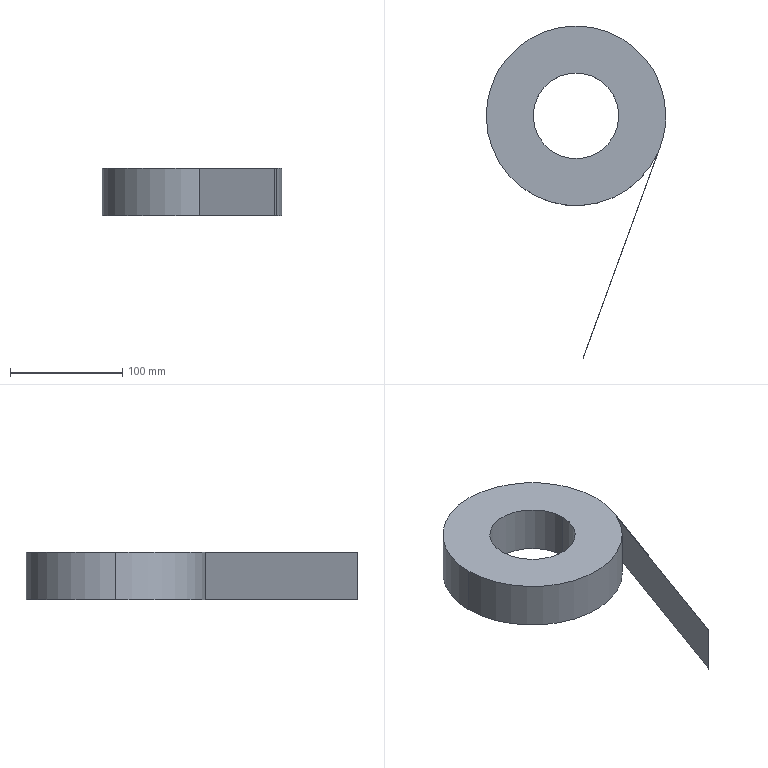Part | STEP file | 10000020479swp000-1 | 1 solid | 10 faces | box 160 x 295.688 x 42 mm | volume 654576 mm3 | cylinder 5 | plane 5 | commonest cylinder face diameters 160 x3 76.2 x2
STEP:
#1=CARTESIAN_POINT('',(-38.1,0.,30.));
#2=VERTEX_POINT('',#1);
#3=CARTESIAN_POINT('',(38.1,0.,30.));
#4=VERTEX_POINT('',#3);
#5=CARTESIAN_POINT('',(0.,0.,30.));
#6=DIRECTION('',(0.,0.,1.));
#7=DIRECTION('',(1.,0.,0.));
#8=AXIS2_PLACEMENT_3D('',#5,#6,#7);
#9=CIRCLE('',#8,38.1);
#10=EDGE_CURVE('',#2,#4,#9,.T.);
#11=ORIENTED_EDGE('',*,*,#10,.T.);
#12=CARTESIAN_POINT('',(38.1,0.,-12.));
#13=VERTEX_POINT('',#12);
#14=CARTESIAN_POINT('',(38.1,0.,30.));
#15=DIRECTION('',(0.,0.,-1.));
#16=VECTOR('',#15,1000.);
#17=LINE('',#14,#16);
#18=EDGE_CURVE('',#4,#13,#17,.T.);
#19=ORIENTED_EDGE('',*,*,#18,.T.);
#20=CARTESIAN_POINT('',(-38.1,0.,-12.));
#21=VERTEX_POINT('',#20);
#22=CARTESIAN_POINT('',(0.,0.,-12.));
#23=DIRECTION('',(0.,0.,1.));
#24=DIRECTION('',(1.,0.,0.));
#25=AXIS2_PLACEMENT_3D('',#22,#23,#24);
#26=CIRCLE('',#25,38.1);
#27=EDGE_CURVE('',#21,#13,#26,.T.);
#28=ORIENTED_EDGE('',*,*,#27,.F.);
#29=CARTESIAN_POINT('',(-38.1,0.,30.));
#30=DIRECTION('',(0.,0.,-1.));
#31=VECTOR('',#30,1000.);
#32=LINE('',#29,#31);
#33=EDGE_CURVE('',#2,#21,#32,.T.);
#34=ORIENTED_EDGE('',*,*,#33,.F.);
#35=EDGE_LOOP('',(#11,#19,#28,#34));
#36=FACE_OUTER_BOUND('',#35,.T.);
#37=CARTESIAN_POINT('',(0.,0.,30.));
#38=DIRECTION('',(0.,0.,-1.));
#39=DIRECTION('',(-1.,0.,0.));
#40=AXIS2_PLACEMENT_3D('',#37,#38,#39);
#41=CYLINDRICAL_SURFACE('',#40,38.1);
#42=ADVANCED_FACE('',(#36),#41,.F.);
#43=CARTESIAN_POINT('',(80.,0.,30.));
#44=VERTEX_POINT('',#43);
#45=CARTESIAN_POINT('',(-80.,0.,30.));
#46=VERTEX_POINT('',#45);
#47=CARTESIAN_POINT('',(0.,0.,30.));
#48=DIRECTION('',(0.,0.,1.));
#49=DIRECTION('',(1.,0.,0.));
#50=AXIS2_PLACEMENT_3D('',#47,#48,#49);
#51=CIRCLE('',#50,80.);
#52=EDGE_CURVE('',#44,#46,#51,.T.);
#53=ORIENTED_EDGE('',*,*,#52,.F.);
#54=CARTESIAN_POINT('',(80.,0.,-12.));
#55=VERTEX_POINT('',#54);
#56=CARTESIAN_POINT('',(80.,0.,30.));
#57=DIRECTION('',(0.,0.,-1.));
#58=VECTOR('',#57,1000.);
#59=LINE('',#56,#58);
#60=EDGE_CURVE('',#44,#55,#59,.T.);
#61=ORIENTED_EDGE('',*,*,#60,.T.);
#62=CARTESIAN_POINT('',(-80.,0.,-12.));
#63=VERTEX_POINT('',#62);
#64=CARTESIAN_POINT('',(0.,0.,-12.));
#65=DIRECTION('',(0.,0.,1.));
#66=DIRECTION('',(1.,0.,0.));
#67=AXIS2_PLACEMENT_3D('',#64,#65,#66);
#68=CIRCLE('',#67,80.);
#69=EDGE_CURVE('',#55,#63,#68,.T.);
#70=ORIENTED_EDGE('',*,*,#69,.T.);
#71=CARTESIAN_POINT('',(-80.,0.,30.));
#72=DIRECTION('',(0.,0.,-1.));
#73=VECTOR('',#72,1000.);
#74=LINE('',#71,#73);
#75=EDGE_CURVE('',#46,#63,#74,.T.);
#76=ORIENTED_EDGE('',*,*,#75,.F.);
#77=EDGE_LOOP('',(#53,#61,#70,#76));
#78=FACE_OUTER_BOUND('',#77,.T.);
#79=CARTESIAN_POINT('',(0.,0.,30.));
#80=DIRECTION('',(0.,0.,-1.));
#81=DIRECTION('',(-1.,0.,0.));
#82=AXIS2_PLACEMENT_3D('',#79,#80,#81);
#83=CYLINDRICAL_SURFACE('',#82,80.);
#84=ADVANCED_FACE('',(#78),#83,.T.);
#85=CARTESIAN_POINT('',(73.054,-32.606,30.));
#86=VERTEX_POINT('',#85);
#87=CARTESIAN_POINT('',(0.,0.,30.));
#88=DIRECTION('',(0.,0.,1.));
#89=DIRECTION('',(1.,0.,0.));
#90=AXIS2_PLACEMENT_3D('',#87,#88,#89);
#91=CIRCLE('',#90,80.);
#92=EDGE_CURVE('',#46,#86,#91,.T.);
#93=ORIENTED_EDGE('',*,*,#92,.F.);
#94=ORIENTED_EDGE('',*,*,#75,.T.);
#95=CARTESIAN_POINT('',(73.054,-32.606,-12.));
#96=VERTEX_POINT('',#95);
#97=CARTESIAN_POINT('',(0.,0.,-12.));
#98=DIRECTION('',(0.,0.,1.));
#99=DIRECTION('',(1.,0.,0.));
#100=AXIS2_PLACEMENT_3D('',#97,#98,#99);
#101=CIRCLE('',#100,80.);
#102=EDGE_CURVE('',#63,#96,#101,.T.);
#103=ORIENTED_EDGE('',*,*,#102,.T.);
#104=CARTESIAN_POINT('',(73.054,-32.606,30.));
#105=DIRECTION('',(0.,0.,1.));
#106=VECTOR('',#105,1000.);
#107=LINE('',#104,#106);
#108=EDGE_CURVE('',#96,#86,#107,.T.);
#109=ORIENTED_EDGE('',*,*,#108,.T.);
#110=EDGE_LOOP('',(#93,#94,#103,#109));
#111=FACE_OUTER_BOUND('',#110,.T.);
#112=CARTESIAN_POINT('',(0.,0.,30.));
#113=DIRECTION('',(0.,0.,-1.));
#114=DIRECTION('',(-1.,0.,0.));
#115=AXIS2_PLACEMENT_3D('',#112,#113,#114);
#116=CYLINDRICAL_SURFACE('',#115,80.);
#117=ADVANCED_FACE('',(#111),#116,.T.);
#118=ORIENTED_EDGE('',*,*,#60,.F.);
#119=CARTESIAN_POINT('',(75.175,-27.362,30.));
#120=VERTEX_POINT('',#119);
#121=CARTESIAN_POINT('',(0.,0.,30.));
#122=DIRECTION('',(0.,0.,1.));
#123=DIRECTION('',(1.,0.,0.));
#124=AXIS2_PLACEMENT_3D('',#121,#122,#123);
#125=CIRCLE('',#124,80.);
#126=EDGE_CURVE('',#120,#44,#125,.T.);
#127=ORIENTED_EDGE('',*,*,#126,.F.);
#128=CARTESIAN_POINT('',(75.175,-27.362,-12.));
#129=VERTEX_POINT('',#128);
#130=CARTESIAN_POINT('',(75.175,-27.362,-200.541));
#131=DIRECTION('',(0.,0.,1.));
#132=VECTOR('',#131,1000.);
#133=LINE('',#130,#132);
#134=EDGE_CURVE('',#129,#120,#133,.T.);
#135=ORIENTED_EDGE('',*,*,#134,.F.);
#136=CARTESIAN_POINT('',(0.,0.,-12.));
#137=DIRECTION('',(0.,0.,1.));
#138=DIRECTION('',(1.,0.,0.));
#139=AXIS2_PLACEMENT_3D('',#136,#137,#138);
#140=CIRCLE('',#139,80.);
#141=EDGE_CURVE('',#129,#55,#140,.T.);
#142=ORIENTED_EDGE('',*,*,#141,.T.);
#143=EDGE_LOOP('',(#118,#127,#135,#142));
#144=FACE_OUTER_BOUND('',#143,.T.);
#145=CARTESIAN_POINT('',(0.,0.,30.));
#146=DIRECTION('',(0.,0.,-1.));
#147=DIRECTION('',(-1.,0.,0.));
#148=AXIS2_PLACEMENT_3D('',#145,#146,#147);
#149=CYLINDRICAL_SURFACE('',#148,80.);
#150=ADVANCED_FACE('',(#144),#149,.T.);
#151=CARTESIAN_POINT('',(6.63,-215.688,30.));
#152=VERTEX_POINT('',#151);
#153=CARTESIAN_POINT('',(75.175,-27.362,30.));
#154=DIRECTION('',(-0.342,-0.9397,0.));
#155=VECTOR('',#154,1000.);
#156=LINE('',#153,#155);
#157=EDGE_CURVE('',#120,#152,#156,.T.);
#158=ORIENTED_EDGE('',*,*,#157,.F.);
#159=ORIENTED_EDGE('',*,*,#126,.T.);
#160=ORIENTED_EDGE('',*,*,#52,.T.);
#161=ORIENTED_EDGE('',*,*,#92,.T.);
#162=CARTESIAN_POINT('',(6.442,-215.619,30.));
#163=VERTEX_POINT('',#162);
#164=CARTESIAN_POINT('',(74.987,-27.293,30.));
#165=DIRECTION('',(-0.342,-0.9397,0.));
#166=VECTOR('',#165,1000.);
#167=LINE('',#164,#166);
#168=EDGE_CURVE('',#86,#163,#167,.T.);
#169=ORIENTED_EDGE('',*,*,#168,.T.);
#170=CARTESIAN_POINT('',(6.63,-215.688,30.));
#171=DIRECTION('',(-0.9397,0.342,0.));
#172=VECTOR('',#171,1000.);
#173=LINE('',#170,#172);
#174=EDGE_CURVE('',#152,#163,#173,.T.);
#175=ORIENTED_EDGE('',*,*,#174,.F.);
#176=EDGE_LOOP('',(#158,#159,#160,#161,#169,#175));
#177=FACE_OUTER_BOUND('',#176,.T.);
#178=ORIENTED_EDGE('',*,*,#10,.F.);
#179=CARTESIAN_POINT('',(0.,0.,30.));
#180=DIRECTION('',(0.,0.,1.));
#181=DIRECTION('',(1.,0.,0.));
#182=AXIS2_PLACEMENT_3D('',#179,#180,#181);
#183=CIRCLE('',#182,38.1);
#184=EDGE_CURVE('',#4,#2,#183,.T.);
#185=ORIENTED_EDGE('',*,*,#184,.F.);
#186=EDGE_LOOP('',(#178,#185));
#187=FACE_BOUND('',#186,.T.);
#188=CARTESIAN_POINT('',(0.,0.,30.));
#189=DIRECTION('',(0.,0.,1.));
#190=DIRECTION('',(1.,0.,0.));
#191=AXIS2_PLACEMENT_3D('',#188,#189,#190);
#192=PLANE('',#191);
#193=ADVANCED_FACE('',(#177,#187),#192,.T.);
#194=ORIENTED_EDGE('',*,*,#141,.F.);
#195=CARTESIAN_POINT('',(6.63,-215.688,-12.));
#196=VERTEX_POINT('',#195);
#197=CARTESIAN_POINT('',(75.175,-27.362,-12.));
#198=DIRECTION('',(0.342,0.9397,0.));
#199=VECTOR('',#198,1000.);
#200=LINE('',#197,#199);
#201=EDGE_CURVE('',#196,#129,#200,.T.);
#202=ORIENTED_EDGE('',*,*,#201,.F.);
#203=CARTESIAN_POINT('',(6.442,-215.619,-12.));
#204=VERTEX_POINT('',#203);
#205=CARTESIAN_POINT('',(6.63,-215.688,-12.));
#206=DIRECTION('',(0.9397,-0.342,0.));
#207=VECTOR('',#206,1000.);
#208=LINE('',#205,#207);
#209=EDGE_CURVE('',#204,#196,#208,.T.);
#210=ORIENTED_EDGE('',*,*,#209,.F.);
#211=CARTESIAN_POINT('',(74.987,-27.293,-12.));
#212=DIRECTION('',(0.342,0.9397,0.));
#213=VECTOR('',#212,1000.);
#214=LINE('',#211,#213);
#215=EDGE_CURVE('',#204,#96,#214,.T.);
#216=ORIENTED_EDGE('',*,*,#215,.T.);
#217=ORIENTED_EDGE('',*,*,#102,.F.);
#218=ORIENTED_EDGE('',*,*,#69,.F.);
#219=EDGE_LOOP('',(#194,#202,#210,#216,#217,#218));
#220=FACE_OUTER_BOUND('',#219,.T.);
#221=ORIENTED_EDGE('',*,*,#27,.T.);
#222=CARTESIAN_POINT('',(0.,0.,-12.));
#223=DIRECTION('',(0.,0.,1.));
#224=DIRECTION('',(1.,0.,0.));
#225=AXIS2_PLACEMENT_3D('',#222,#223,#224);
#226=CIRCLE('',#225,38.1);
#227=EDGE_CURVE('',#13,#21,#226,.T.);
#228=ORIENTED_EDGE('',*,*,#227,.T.);
#229=EDGE_LOOP('',(#221,#228));
#230=FACE_BOUND('',#229,.T.);
#231=CARTESIAN_POINT('',(0.,0.,-12.));
#232=DIRECTION('',(0.,0.,1.));
#233=DIRECTION('',(1.,0.,0.));
#234=AXIS2_PLACEMENT_3D('',#231,#232,#233);
#235=PLANE('',#234);
#236=ADVANCED_FACE('',(#220,#230),#235,.F.);
#237=ORIENTED_EDGE('',*,*,#18,.F.);
#238=ORIENTED_EDGE('',*,*,#184,.T.);
#239=ORIENTED_EDGE('',*,*,#33,.T.);
#240=ORIENTED_EDGE('',*,*,#227,.F.);
#241=EDGE_LOOP('',(#237,#238,#239,#240));
#242=FACE_OUTER_BOUND('',#241,.T.);
#243=CARTESIAN_POINT('',(0.,0.,30.));
#244=DIRECTION('',(0.,0.,-1.));
#245=DIRECTION('',(-1.,0.,0.));
#246=AXIS2_PLACEMENT_3D('',#243,#244,#245);
#247=CYLINDRICAL_SURFACE('',#246,38.1);
#248=ADVANCED_FACE('',(#242),#247,.F.);
#249=ORIENTED_EDGE('',*,*,#108,.F.);
#250=ORIENTED_EDGE('',*,*,#215,.F.);
#251=CARTESIAN_POINT('',(6.442,-215.619,-200.541));
#252=DIRECTION('',(0.,0.,1.));
#253=VECTOR('',#252,1000.);
#254=LINE('',#251,#253);
#255=EDGE_CURVE('',#204,#163,#254,.T.);
#256=ORIENTED_EDGE('',*,*,#255,.T.);
#257=ORIENTED_EDGE('',*,*,#168,.F.);
#258=EDGE_LOOP('',(#249,#250,#256,#257));
#259=FACE_OUTER_BOUND('',#258,.T.);
#260=CARTESIAN_POINT('',(74.987,-27.293,-200.541));
#261=DIRECTION('',(-0.9397,0.342,0.));
#262=DIRECTION('',(-0.342,-0.9397,0.));
#263=AXIS2_PLACEMENT_3D('',#260,#261,#262);
#264=PLANE('',#263);
#265=ADVANCED_FACE('',(#259),#264,.T.);
#266=ORIENTED_EDGE('',*,*,#255,.F.);
#267=ORIENTED_EDGE('',*,*,#209,.T.);
#268=CARTESIAN_POINT('',(6.63,-215.688,-200.541));
#269=DIRECTION('',(0.,0.,1.));
#270=VECTOR('',#269,1000.);
#271=LINE('',#268,#270);
#272=EDGE_CURVE('',#196,#152,#271,.T.);
#273=ORIENTED_EDGE('',*,*,#272,.T.);
#274=ORIENTED_EDGE('',*,*,#174,.T.);
#275=EDGE_LOOP('',(#266,#267,#273,#274));
#276=FACE_OUTER_BOUND('',#275,.T.);
#277=CARTESIAN_POINT('',(6.63,-215.688,-200.541));
#278=DIRECTION('',(0.342,0.9397,0.));
#279=DIRECTION('',(-0.9397,0.342,0.));
#280=AXIS2_PLACEMENT_3D('',#277,#278,#279);
#281=PLANE('',#280);
#282=ADVANCED_FACE('',(#276),#281,.F.);
#283=ORIENTED_EDGE('',*,*,#272,.F.);
#284=ORIENTED_EDGE('',*,*,#201,.T.);
#285=ORIENTED_EDGE('',*,*,#134,.T.);
#286=ORIENTED_EDGE('',*,*,#157,.T.);
#287=EDGE_LOOP('',(#283,#284,#285,#286));
#288=FACE_OUTER_BOUND('',#287,.T.);
#289=CARTESIAN_POINT('',(75.175,-27.362,-200.541));
#290=DIRECTION('',(-0.9397,0.342,0.));
#291=DIRECTION('',(-0.342,-0.9397,0.));
#292=AXIS2_PLACEMENT_3D('',#289,#290,#291);
#293=PLANE('',#292);
#294=ADVANCED_FACE('',(#288),#293,.F.);
#295=CLOSED_SHELL('',(#42,#84,#117,#150,#193,#236,#248,#265,#282,#294));
#296=MANIFOLD_SOLID_BREP('',#295);
#297=CARTESIAN_POINT('',(0.,0.,0.));
#298=DIRECTION('',(0.,0.,1.));
#299=DIRECTION('',(1.,0.,0.));
#300=AXIS2_PLACEMENT_3D('',#297,#298,#299);
#301=(LENGTH_UNIT()NAMED_UNIT(*)SI_UNIT(.MILLI.,.METRE.));
#302=UNCERTAINTY_MEASURE_WITH_UNIT(LENGTH_MEASURE(0.00001),#301,'','');
#303=(NAMED_UNIT(*)PLANE_ANGLE_UNIT()SI_UNIT($,.RADIAN.));
#304=(NAMED_UNIT(*)SI_UNIT($,.STERADIAN.)SOLID_ANGLE_UNIT());
#305=(GEOMETRIC_REPRESENTATION_CONTEXT(3)GLOBAL_UNCERTAINTY_ASSIGNED_CONTEXT((#302))GLOBAL_UNIT_ASSIGNED_CONTEXT((#301,#303,#304))REPRESENTATION_CONTEXT('',''));
#306=ADVANCED_BREP_SHAPE_REPRESENTATION('',(#296,#300),#305);